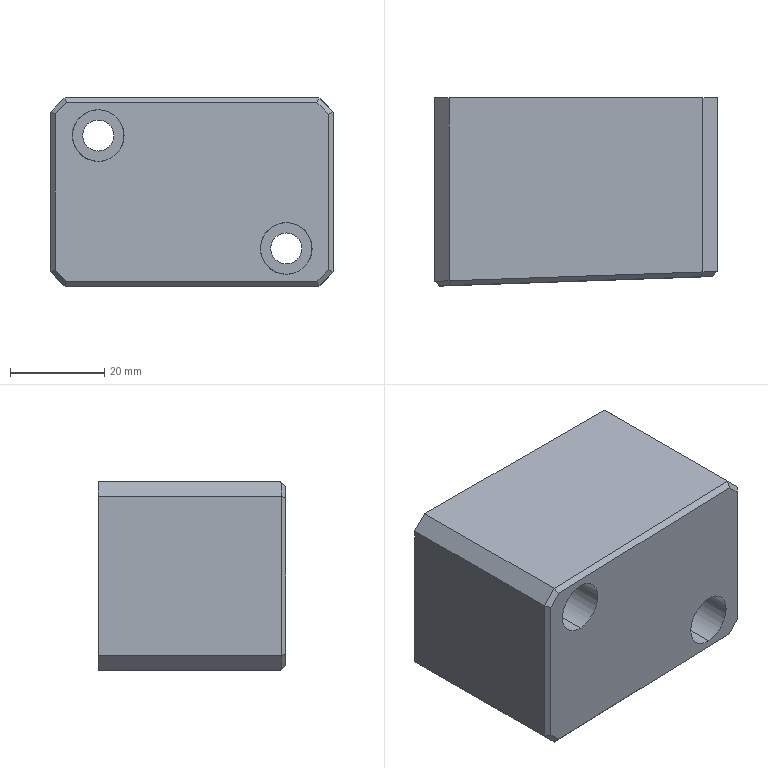Part | SolidWorks | features HoleWzd 3, Chamfer 2, Extrusion 1 | 1 solid | 36 faces | box 60 x 39.966 x 40 mm | volume 86382 mm3 | plane 20 | cylinder 12 | cone 4 | commonest cylinder face diameters 6.6 x4 8 x4 11 x4
STEP:
#1=CARTESIAN_POINT('',(-27.515,48.13,4.));
#2=VERTEX_POINT('',#1);
#3=CARTESIAN_POINT('',(-27.515,48.13,12.));
#4=VERTEX_POINT('',#3);
#5=CARTESIAN_POINT('',(-27.515,48.13,8.));
#6=DIRECTION('',(0.,1.,0.));
#7=DIRECTION('',(0.,0.,1.));
#8=AXIS2_PLACEMENT_3D('',#5,#6,#7);
#9=CIRCLE('',#8,4.);
#10=EDGE_CURVE('',#2,#4,#9,.T.);
#11=ORIENTED_EDGE('',*,*,#10,.F.);
#12=CARTESIAN_POINT('',(-27.515,60.63,4.));
#13=VERTEX_POINT('',#12);
#14=CARTESIAN_POINT('',(-27.515,60.63,4.));
#15=DIRECTION('',(0.,1.,0.));
#16=VECTOR('',#15,1000.);
#17=LINE('',#14,#16);
#18=EDGE_CURVE('',#2,#13,#17,.T.);
#19=ORIENTED_EDGE('',*,*,#18,.T.);
#20=CARTESIAN_POINT('',(-27.515,60.63,12.));
#21=VERTEX_POINT('',#20);
#22=CARTESIAN_POINT('',(-27.515,60.63,8.));
#23=DIRECTION('',(0.,1.,0.));
#24=DIRECTION('',(0.,0.,1.));
#25=AXIS2_PLACEMENT_3D('',#22,#23,#24);
#26=CIRCLE('',#25,4.);
#27=EDGE_CURVE('',#13,#21,#26,.T.);
#28=ORIENTED_EDGE('',*,*,#27,.T.);
#29=CARTESIAN_POINT('',(-27.515,60.63,12.));
#30=DIRECTION('',(0.,1.,0.));
#31=VECTOR('',#30,1000.);
#32=LINE('',#29,#31);
#33=EDGE_CURVE('',#4,#21,#32,.T.);
#34=ORIENTED_EDGE('',*,*,#33,.F.);
#35=EDGE_LOOP('',(#11,#19,#28,#34));
#36=FACE_OUTER_BOUND('',#35,.T.);
#37=CARTESIAN_POINT('',(-27.515,60.63,8.));
#38=DIRECTION('',(0.,1.,0.));
#39=DIRECTION('',(0.,0.,1.));
#40=AXIS2_PLACEMENT_3D('',#37,#38,#39);
#41=CYLINDRICAL_SURFACE('',#40,4.);
#42=ADVANCED_FACE('',(#36),#41,.F.);
#43=CARTESIAN_POINT('',(-27.515,45.727,8.));
#44=VERTEX_POINT('',#43);
#45=CARTESIAN_POINT('',(-27.515,48.13,12.));
#46=DIRECTION('',(0.,0.515,0.8572));
#47=VECTOR('',#46,1000.);
#48=LINE('',#45,#47);
#49=EDGE_CURVE('',#44,#4,#48,.T.);
#50=ORIENTED_EDGE('',*,*,#49,.F.);
#51=CARTESIAN_POINT('',(-27.515,48.13,4.));
#52=DIRECTION('',(0.,0.515,-0.8572));
#53=VECTOR('',#52,1000.);
#54=LINE('',#51,#53);
#55=EDGE_CURVE('',#44,#2,#54,.T.);
#56=ORIENTED_EDGE('',*,*,#55,.T.);
#57=ORIENTED_EDGE('',*,*,#10,.T.);
#58=EDGE_LOOP('',(#50,#56,#57));
#59=FACE_OUTER_BOUND('',#58,.T.);
#60=CARTESIAN_POINT('',(-27.515,48.13,8.));
#61=DIRECTION('',(0.,1.,0.));
#62=DIRECTION('',(0.,0.,1.));
#63=AXIS2_PLACEMENT_3D('',#60,#61,#62);
#64=CONICAL_SURFACE('',#63,4.,1.03);
#65=ADVANCED_FACE('',(#59),#64,.F.);
#66=CARTESIAN_POINT('',(12.461,48.13,28.));
#67=VERTEX_POINT('',#66);
#68=CARTESIAN_POINT('',(12.461,48.13,36.));
#69=VERTEX_POINT('',#68);
#70=CARTESIAN_POINT('',(12.461,48.13,32.));
#71=DIRECTION('',(0.,1.,0.));
#72=DIRECTION('',(0.,0.,1.));
#73=AXIS2_PLACEMENT_3D('',#70,#71,#72);
#74=CIRCLE('',#73,4.);
#75=EDGE_CURVE('',#67,#69,#74,.T.);
#76=ORIENTED_EDGE('',*,*,#75,.F.);
#77=CARTESIAN_POINT('',(12.461,60.63,28.));
#78=VERTEX_POINT('',#77);
#79=CARTESIAN_POINT('',(12.461,60.63,28.));
#80=DIRECTION('',(0.,1.,0.));
#81=VECTOR('',#80,1000.);
#82=LINE('',#79,#81);
#83=EDGE_CURVE('',#67,#78,#82,.T.);
#84=ORIENTED_EDGE('',*,*,#83,.T.);
#85=CARTESIAN_POINT('',(12.461,60.63,36.));
#86=VERTEX_POINT('',#85);
#87=CARTESIAN_POINT('',(12.461,60.63,32.));
#88=DIRECTION('',(0.,1.,0.));
#89=DIRECTION('',(0.,0.,1.));
#90=AXIS2_PLACEMENT_3D('',#87,#88,#89);
#91=CIRCLE('',#90,4.);
#92=EDGE_CURVE('',#78,#86,#91,.T.);
#93=ORIENTED_EDGE('',*,*,#92,.T.);
#94=CARTESIAN_POINT('',(12.461,60.63,36.));
#95=DIRECTION('',(0.,1.,0.));
#96=VECTOR('',#95,1000.);
#97=LINE('',#94,#96);
#98=EDGE_CURVE('',#69,#86,#97,.T.);
#99=ORIENTED_EDGE('',*,*,#98,.F.);
#100=EDGE_LOOP('',(#76,#84,#93,#99));
#101=FACE_OUTER_BOUND('',#100,.T.);
#102=CARTESIAN_POINT('',(12.461,60.63,32.));
#103=DIRECTION('',(0.,1.,0.));
#104=DIRECTION('',(0.,0.,1.));
#105=AXIS2_PLACEMENT_3D('',#102,#103,#104);
#106=CYLINDRICAL_SURFACE('',#105,4.);
#107=ADVANCED_FACE('',(#101),#106,.F.);
#108=CARTESIAN_POINT('',(12.461,45.727,32.));
#109=VERTEX_POINT('',#108);
#110=CARTESIAN_POINT('',(12.461,48.13,36.));
#111=DIRECTION('',(0.,0.515,0.8572));
#112=VECTOR('',#111,1000.);
#113=LINE('',#110,#112);
#114=EDGE_CURVE('',#109,#69,#113,.T.);
#115=ORIENTED_EDGE('',*,*,#114,.F.);
#116=CARTESIAN_POINT('',(12.461,48.13,28.));
#117=DIRECTION('',(0.,0.515,-0.8572));
#118=VECTOR('',#117,1000.);
#119=LINE('',#116,#118);
#120=EDGE_CURVE('',#109,#67,#119,.T.);
#121=ORIENTED_EDGE('',*,*,#120,.T.);
#122=ORIENTED_EDGE('',*,*,#75,.T.);
#123=EDGE_LOOP('',(#115,#121,#122));
#124=FACE_OUTER_BOUND('',#123,.T.);
#125=CARTESIAN_POINT('',(12.461,48.13,32.));
#126=DIRECTION('',(0.,1.,0.));
#127=DIRECTION('',(0.,0.,1.));
#128=AXIS2_PLACEMENT_3D('',#125,#126,#127);
#129=CONICAL_SURFACE('',#128,4.,1.03);
#130=ADVANCED_FACE('',(#124),#129,.F.);
#131=CARTESIAN_POINT('',(-27.515,20.982,26.5));
#132=VERTEX_POINT('',#131);
#133=CARTESIAN_POINT('',(-27.515,20.982,37.5));
#134=VERTEX_POINT('',#133);
#135=CARTESIAN_POINT('',(-27.515,20.982,26.5));
#136=CARTESIAN_POINT('',(-38.515,20.597,26.5));
#137=CARTESIAN_POINT('',(-38.515,20.597,37.5));
#138=CARTESIAN_POINT('',(-27.515,20.982,37.5));
#139=(BOUNDED_CURVE()B_SPLINE_CURVE(3,(#135,#136,#137,#138),.UNSPECIFIED.,.F.,.F.)B_SPLINE_CURVE_WITH_KNOTS((4,4),(1.571,4.712),.UNSPECIFIED.)CURVE()GEOMETRIC_REPRESENTATION_ITEM()RATIONAL_B_SPLINE_CURVE((1.,0.3333,0.3333,1.))REPRESENTATION_ITEM(''));
#140=EDGE_CURVE('',#132,#134,#139,.T.);
#141=ORIENTED_EDGE('',*,*,#140,.F.);
#142=CARTESIAN_POINT('',(-27.515,40.63,26.5));
#143=VERTEX_POINT('',#142);
#144=CARTESIAN_POINT('',(-27.515,40.63,26.5));
#145=DIRECTION('',(0.,1.,0.));
#146=VECTOR('',#145,1000.);
#147=LINE('',#144,#146);
#148=EDGE_CURVE('',#132,#143,#147,.T.);
#149=ORIENTED_EDGE('',*,*,#148,.T.);
#150=CARTESIAN_POINT('',(-27.515,40.63,37.5));
#151=VERTEX_POINT('',#150);
#152=CARTESIAN_POINT('',(-27.515,40.63,32.));
#153=DIRECTION('',(0.,1.,0.));
#154=DIRECTION('',(0.,0.,1.));
#155=AXIS2_PLACEMENT_3D('',#152,#153,#154);
#156=CIRCLE('',#155,5.5);
#157=EDGE_CURVE('',#143,#151,#156,.T.);
#158=ORIENTED_EDGE('',*,*,#157,.T.);
#159=CARTESIAN_POINT('',(-27.515,40.63,37.5));
#160=DIRECTION('',(0.,1.,0.));
#161=VECTOR('',#160,1000.);
#162=LINE('',#159,#161);
#163=EDGE_CURVE('',#134,#151,#162,.T.);
#164=ORIENTED_EDGE('',*,*,#163,.F.);
#165=EDGE_LOOP('',(#141,#149,#158,#164));
#166=FACE_OUTER_BOUND('',#165,.T.);
#167=CARTESIAN_POINT('',(-27.515,40.63,32.));
#168=DIRECTION('',(0.,1.,0.));
#169=DIRECTION('',(0.,0.,1.));
#170=AXIS2_PLACEMENT_3D('',#167,#168,#169);
#171=CYLINDRICAL_SURFACE('',#170,5.5);
#172=ADVANCED_FACE('',(#166),#171,.F.);
#173=CARTESIAN_POINT('',(12.461,22.378,2.5));
#174=VERTEX_POINT('',#173);
#175=CARTESIAN_POINT('',(12.461,22.378,13.5));
#176=VERTEX_POINT('',#175);
#177=CARTESIAN_POINT('',(12.461,22.378,2.5));
#178=CARTESIAN_POINT('',(1.461,21.993,2.5));
#179=CARTESIAN_POINT('',(1.461,21.993,13.5));
#180=CARTESIAN_POINT('',(12.461,22.378,13.5));
#181=(BOUNDED_CURVE()B_SPLINE_CURVE(3,(#177,#178,#179,#180),.UNSPECIFIED.,.F.,.F.)B_SPLINE_CURVE_WITH_KNOTS((4,4),(1.571,4.712),.UNSPECIFIED.)CURVE()GEOMETRIC_REPRESENTATION_ITEM()RATIONAL_B_SPLINE_CURVE((1.,0.3333,0.3333,1.))REPRESENTATION_ITEM(''));
#182=EDGE_CURVE('',#174,#176,#181,.T.);
#183=ORIENTED_EDGE('',*,*,#182,.F.);
#184=CARTESIAN_POINT('',(12.461,40.63,2.5));
#185=VERTEX_POINT('',#184);
#186=CARTESIAN_POINT('',(12.461,40.63,2.5));
#187=DIRECTION('',(0.,1.,0.));
#188=VECTOR('',#187,1000.);
#189=LINE('',#186,#188);
#190=EDGE_CURVE('',#174,#185,#189,.T.);
#191=ORIENTED_EDGE('',*,*,#190,.T.);
#192=CARTESIAN_POINT('',(12.461,40.63,13.5));
#193=VERTEX_POINT('',#192);
#194=CARTESIAN_POINT('',(12.461,40.63,8.));
#195=DIRECTION('',(0.,1.,0.));
#196=DIRECTION('',(0.,0.,1.));
#197=AXIS2_PLACEMENT_3D('',#194,#195,#196);
#198=CIRCLE('',#197,5.5);
#199=EDGE_CURVE('',#185,#193,#198,.T.);
#200=ORIENTED_EDGE('',*,*,#199,.T.);
#201=CARTESIAN_POINT('',(12.461,40.63,13.5));
#202=DIRECTION('',(0.,1.,0.));
#203=VECTOR('',#202,1000.);
#204=LINE('',#201,#203);
#205=EDGE_CURVE('',#176,#193,#204,.T.);
#206=ORIENTED_EDGE('',*,*,#205,.F.);
#207=EDGE_LOOP('',(#183,#191,#200,#206));
#208=FACE_OUTER_BOUND('',#207,.T.);
#209=CARTESIAN_POINT('',(12.461,40.63,8.));
#210=DIRECTION('',(0.,1.,0.));
#211=DIRECTION('',(0.,0.,1.));
#212=AXIS2_PLACEMENT_3D('',#209,#210,#211);
#213=CYLINDRICAL_SURFACE('',#212,5.5);
#214=ADVANCED_FACE('',(#208),#213,.F.);
#215=CARTESIAN_POINT('',(-27.515,40.63,35.3));
#216=VERTEX_POINT('',#215);
#217=CARTESIAN_POINT('',(-27.515,40.63,28.7));
#218=VERTEX_POINT('',#217);
#219=CARTESIAN_POINT('',(-27.515,40.63,32.));
#220=DIRECTION('',(0.,-1.,0.));
#221=DIRECTION('',(0.,0.,1.));
#222=AXIS2_PLACEMENT_3D('',#219,#220,#221);
#223=CIRCLE('',#222,3.3);
#224=EDGE_CURVE('',#216,#218,#223,.T.);
#225=ORIENTED_EDGE('',*,*,#224,.T.);
#226=CARTESIAN_POINT('',(-27.515,60.63,28.7));
#227=VERTEX_POINT('',#226);
#228=CARTESIAN_POINT('',(-27.515,60.63,28.7));
#229=DIRECTION('',(0.,1.,0.));
#230=VECTOR('',#229,1000.);
#231=LINE('',#228,#230);
#232=EDGE_CURVE('',#218,#227,#231,.T.);
#233=ORIENTED_EDGE('',*,*,#232,.T.);
#234=CARTESIAN_POINT('',(-27.515,60.63,35.3));
#235=VERTEX_POINT('',#234);
#236=CARTESIAN_POINT('',(-27.515,60.63,32.));
#237=DIRECTION('',(0.,1.,0.));
#238=DIRECTION('',(0.,0.,1.));
#239=AXIS2_PLACEMENT_3D('',#236,#237,#238);
#240=CIRCLE('',#239,3.3);
#241=EDGE_CURVE('',#227,#235,#240,.T.);
#242=ORIENTED_EDGE('',*,*,#241,.T.);
#243=CARTESIAN_POINT('',(-27.515,60.63,35.3));
#244=DIRECTION('',(0.,1.,0.));
#245=VECTOR('',#244,1000.);
#246=LINE('',#243,#245);
#247=EDGE_CURVE('',#216,#235,#246,.T.);
#248=ORIENTED_EDGE('',*,*,#247,.F.);
#249=EDGE_LOOP('',(#225,#233,#242,#248));
#250=FACE_OUTER_BOUND('',#249,.T.);
#251=CARTESIAN_POINT('',(-27.515,60.63,32.));
#252=DIRECTION('',(0.,1.,0.));
#253=DIRECTION('',(0.,0.,1.));
#254=AXIS2_PLACEMENT_3D('',#251,#252,#253);
#255=CYLINDRICAL_SURFACE('',#254,3.3);
#256=ADVANCED_FACE('',(#250),#255,.F.);
#257=CARTESIAN_POINT('',(12.461,40.63,11.3));
#258=VERTEX_POINT('',#257);
#259=CARTESIAN_POINT('',(12.461,40.63,4.7));
#260=VERTEX_POINT('',#259);
#261=CARTESIAN_POINT('',(12.461,40.63,8.));
#262=DIRECTION('',(0.,-1.,0.));
#263=DIRECTION('',(0.,0.,1.));
#264=AXIS2_PLACEMENT_3D('',#261,#262,#263);
#265=CIRCLE('',#264,3.3);
#266=EDGE_CURVE('',#258,#260,#265,.T.);
#267=ORIENTED_EDGE('',*,*,#266,.T.);
#268=CARTESIAN_POINT('',(12.461,60.63,4.7));
#269=VERTEX_POINT('',#268);
#270=CARTESIAN_POINT('',(12.461,60.63,4.7));
#271=DIRECTION('',(0.,1.,0.));
#272=VECTOR('',#271,1000.);
#273=LINE('',#270,#272);
#274=EDGE_CURVE('',#260,#269,#273,.T.);
#275=ORIENTED_EDGE('',*,*,#274,.T.);
#276=CARTESIAN_POINT('',(12.461,60.63,11.3));
#277=VERTEX_POINT('',#276);
#278=CARTESIAN_POINT('',(12.461,60.63,8.));
#279=DIRECTION('',(0.,1.,0.));
#280=DIRECTION('',(0.,0.,1.));
#281=AXIS2_PLACEMENT_3D('',#278,#279,#280);
#282=CIRCLE('',#281,3.3);
#283=EDGE_CURVE('',#269,#277,#282,.T.);
#284=ORIENTED_EDGE('',*,*,#283,.T.);
#285=CARTESIAN_POINT('',(12.461,60.63,11.3));
#286=DIRECTION('',(0.,1.,0.));
#287=VECTOR('',#286,1000.);
#288=LINE('',#285,#287);
#289=EDGE_CURVE('',#258,#277,#288,.T.);
#290=ORIENTED_EDGE('',*,*,#289,.F.);
#291=EDGE_LOOP('',(#267,#275,#284,#290));
#292=FACE_OUTER_BOUND('',#291,.T.);
#293=CARTESIAN_POINT('',(12.461,60.63,8.));
#294=DIRECTION('',(0.,1.,0.));
#295=DIRECTION('',(0.,0.,1.));
#296=AXIS2_PLACEMENT_3D('',#293,#294,#295);
#297=CYLINDRICAL_SURFACE('',#296,3.3);
#298=ADVANCED_FACE('',(#292),#297,.F.);
#299=CARTESIAN_POINT('',(-37.581,60.63,3.));
#300=VERTEX_POINT('',#299);
#301=CARTESIAN_POINT('',(-37.581,21.63,3.));
#302=VERTEX_POINT('',#301);
#303=CARTESIAN_POINT('',(-37.581,60.63,3.));
#304=DIRECTION('',(0.,-1.,0.));
#305=VECTOR('',#304,1000.);
#306=LINE('',#303,#305);
#307=EDGE_CURVE('',#300,#302,#306,.T.);
#308=ORIENTED_EDGE('',*,*,#307,.T.);
#309=CARTESIAN_POINT('',(-37.581,21.63,3.));
#310=VERTEX_POINT('',#309);
#311=CARTESIAN_POINT('',(-37.581,11.958,16.345));
#312=DIRECTION('',(0.,-0.5869,0.8097));
#313=VECTOR('',#312,1000.);
#314=LINE('',#311,#313);
#315=EDGE_CURVE('',#302,#310,#314,.T.);
#316=ORIENTED_EDGE('',*,*,#315,.T.);
#317=CARTESIAN_POINT('',(-37.581,21.63,37.));
#318=VERTEX_POINT('',#317);
#319=CARTESIAN_POINT('',(-37.581,21.63,40.));
#320=DIRECTION('',(0.,0.,1.));
#321=VECTOR('',#320,1000.);
#322=LINE('',#319,#321);
#323=EDGE_CURVE('',#310,#318,#322,.T.);
#324=ORIENTED_EDGE('',*,*,#323,.T.);
#325=CARTESIAN_POINT('',(-37.581,21.63,37.));
#326=VERTEX_POINT('',#325);
#327=CARTESIAN_POINT('',(-37.581,21.696,37.091));
#328=DIRECTION('',(0.,0.5869,0.8097));
#329=VECTOR('',#328,1000.);
#330=LINE('',#327,#329);
#331=EDGE_CURVE('',#318,#326,#330,.T.);
#332=ORIENTED_EDGE('',*,*,#331,.T.);
#333=CARTESIAN_POINT('',(-37.581,60.63,37.));
#334=VERTEX_POINT('',#333);
#335=CARTESIAN_POINT('',(-37.581,60.63,37.));
#336=DIRECTION('',(0.,1.,0.));
#337=VECTOR('',#336,1000.);
#338=LINE('',#335,#337);
#339=EDGE_CURVE('',#326,#334,#338,.T.);
#340=ORIENTED_EDGE('',*,*,#339,.T.);
#341=CARTESIAN_POINT('',(-37.581,60.63,40.));
#342=DIRECTION('',(0.,0.,-1.));
#343=VECTOR('',#342,1000.);
#344=LINE('',#341,#343);
#345=EDGE_CURVE('',#334,#300,#344,.T.);
#346=ORIENTED_EDGE('',*,*,#345,.T.);
#347=EDGE_LOOP('',(#308,#316,#324,#332,#340,#346));
#348=FACE_OUTER_BOUND('',#347,.T.);
#349=CARTESIAN_POINT('',(-37.581,60.63,40.));
#350=DIRECTION('',(1.,0.,0.));
#351=DIRECTION('',(0.,1.,0.));
#352=AXIS2_PLACEMENT_3D('',#349,#350,#351);
#353=PLANE('',#352);
#354=ADVANCED_FACE('',(#348),#353,.F.);
#355=CARTESIAN_POINT('',(-27.515,20.982,37.5));
#356=CARTESIAN_POINT('',(-16.515,21.366,37.5));
#357=CARTESIAN_POINT('',(-16.515,21.366,26.5));
#358=CARTESIAN_POINT('',(-27.515,20.982,26.5));
#359=(BOUNDED_CURVE()B_SPLINE_CURVE(3,(#355,#356,#357,#358),.UNSPECIFIED.,.F.,.T.)B_SPLINE_CURVE_WITH_KNOTS((4,4),(4.712,7.854),.UNSPECIFIED.)CURVE()GEOMETRIC_REPRESENTATION_ITEM()RATIONAL_B_SPLINE_CURVE((1.,0.3333,0.3333,1.))REPRESENTATION_ITEM(''));
#360=EDGE_CURVE('',#134,#132,#359,.T.);
#361=ORIENTED_EDGE('',*,*,#360,.T.);
#362=ORIENTED_EDGE('',*,*,#140,.T.);
#363=EDGE_LOOP('',(#361,#362));
#364=FACE_BOUND('',#363,.T.);
#365=CARTESIAN_POINT('',(12.461,22.378,13.5));
#366=CARTESIAN_POINT('',(23.461,22.762,13.5));
#367=CARTESIAN_POINT('',(23.461,22.762,2.5));
#368=CARTESIAN_POINT('',(12.461,22.378,2.5));
#369=(BOUNDED_CURVE()B_SPLINE_CURVE(3,(#365,#366,#367,#368),.UNSPECIFIED.,.F.,.T.)B_SPLINE_CURVE_WITH_KNOTS((4,4),(4.712,7.854),.UNSPECIFIED.)CURVE()GEOMETRIC_REPRESENTATION_ITEM()RATIONAL_B_SPLINE_CURVE((1.,0.3333,0.3333,1.))REPRESENTATION_ITEM(''));
#370=EDGE_CURVE('',#176,#174,#369,.T.);
#371=ORIENTED_EDGE('',*,*,#370,.T.);
#372=ORIENTED_EDGE('',*,*,#182,.T.);
#373=EDGE_LOOP('',(#371,#372));
#374=FACE_BOUND('',#373,.T.);
#375=CARTESIAN_POINT('',(21.419,22.69,3.451));
#376=VERTEX_POINT('',#375);
#377=CARTESIAN_POINT('',(21.419,22.69,36.549));
#378=VERTEX_POINT('',#377);
#379=CARTESIAN_POINT('',(21.419,22.69,40.));
#380=DIRECTION('',(0.,0.,1.));
#381=VECTOR('',#380,1000.);
#382=LINE('',#379,#381);
#383=EDGE_CURVE('',#376,#378,#382,.T.);
#384=ORIENTED_EDGE('',*,*,#383,.T.);
#385=CARTESIAN_POINT('',(18.969,22.605,39.));
#386=VERTEX_POINT('',#385);
#387=CARTESIAN_POINT('',(18.694,22.595,39.275));
#388=DIRECTION('',(-0.7069,-0.02469,0.7069));
#389=VECTOR('',#388,1000.);
#390=LINE('',#387,#389);
#391=EDGE_CURVE('',#378,#386,#390,.T.);
#392=ORIENTED_EDGE('',*,*,#391,.T.);
#393=CARTESIAN_POINT('',(-34.201,20.748,39.));
#394=VERTEX_POINT('',#393);
#395=CARTESIAN_POINT('',(-34.581,20.735,39.));
#396=DIRECTION('',(-0.9994,-0.0349,0.));
#397=VECTOR('',#396,1000.);
#398=LINE('',#395,#397);
#399=EDGE_CURVE('',#386,#394,#398,.T.);
#400=ORIENTED_EDGE('',*,*,#399,.T.);
#401=CARTESIAN_POINT('',(-36.615,20.664,36.586));
#402=VERTEX_POINT('',#401);
#403=CARTESIAN_POINT('',(-36.892,20.654,36.31));
#404=DIRECTION('',(-0.7069,-0.02469,-0.7069));
#405=VECTOR('',#404,1000.);
#406=LINE('',#403,#405);
#407=EDGE_CURVE('',#394,#402,#406,.T.);
#408=ORIENTED_EDGE('',*,*,#407,.T.);
#409=CARTESIAN_POINT('',(-36.615,20.664,3.414));
#410=VERTEX_POINT('',#409);
#411=CARTESIAN_POINT('',(-36.615,20.664,40.));
#412=DIRECTION('',(0.,0.,-1.));
#413=VECTOR('',#412,1000.);
#414=LINE('',#411,#413);
#415=EDGE_CURVE('',#402,#410,#414,.T.);
#416=ORIENTED_EDGE('',*,*,#415,.T.);
#417=CARTESIAN_POINT('',(-34.201,20.748,1.));
#418=VERTEX_POINT('',#417);
#419=CARTESIAN_POINT('',(-33.892,20.759,0.6905));
#420=DIRECTION('',(0.7069,0.02469,-0.7069));
#421=VECTOR('',#420,1000.);
#422=LINE('',#419,#421);
#423=EDGE_CURVE('',#410,#418,#422,.T.);
#424=ORIENTED_EDGE('',*,*,#423,.T.);
#425=CARTESIAN_POINT('',(18.969,22.605,1.));
#426=VERTEX_POINT('',#425);
#427=CARTESIAN_POINT('',(-37.581,20.63,1.));
#428=DIRECTION('',(0.9994,0.0349,0.));
#429=VECTOR('',#428,1000.);
#430=LINE('',#427,#429);
#431=EDGE_CURVE('',#418,#426,#430,.T.);
#432=ORIENTED_EDGE('',*,*,#431,.T.);
#433=CARTESIAN_POINT('',(21.694,22.7,3.725));
#434=DIRECTION('',(0.7069,0.02469,0.7069));
#435=VECTOR('',#434,1000.);
#436=LINE('',#433,#435);
#437=EDGE_CURVE('',#426,#376,#436,.T.);
#438=ORIENTED_EDGE('',*,*,#437,.T.);
#439=EDGE_LOOP('',(#384,#392,#400,#408,#416,#424,#432,#438));
#440=FACE_OUTER_BOUND('',#439,.T.);
#441=CARTESIAN_POINT('',(-37.581,20.63,40.));
#442=DIRECTION('',(-0.0349,0.9994,0.));
#443=DIRECTION('',(-0.9994,-0.0349,0.));
#444=AXIS2_PLACEMENT_3D('',#441,#442,#443);
#445=PLANE('',#444);
#446=ADVANCED_FACE('',(#364,#374,#440),#445,.F.);
#447=CARTESIAN_POINT('',(22.419,60.63,37.));
#448=VERTEX_POINT('',#447);
#449=CARTESIAN_POINT('',(22.419,23.762,37.));
#450=VERTEX_POINT('',#449);
#451=CARTESIAN_POINT('',(22.419,22.725,37.));
#452=DIRECTION('',(0.,-1.,0.));
#453=VECTOR('',#452,1000.);
#454=LINE('',#451,#453);
#455=EDGE_CURVE('',#448,#450,#454,.T.);
#456=ORIENTED_EDGE('',*,*,#455,.T.);
#457=CARTESIAN_POINT('',(22.419,23.762,3.));
#458=VERTEX_POINT('',#457);
#459=CARTESIAN_POINT('',(22.419,23.762,40.));
#460=DIRECTION('',(0.,0.,-1.));
#461=VECTOR('',#460,1000.);
#462=LINE('',#459,#461);
#463=EDGE_CURVE('',#450,#458,#462,.T.);
#464=ORIENTED_EDGE('',*,*,#463,.T.);
#465=CARTESIAN_POINT('',(22.419,60.63,3.));
#466=VERTEX_POINT('',#465);
#467=CARTESIAN_POINT('',(22.419,60.63,3.));
#468=DIRECTION('',(0.,1.,0.));
#469=VECTOR('',#468,1000.);
#470=LINE('',#467,#469);
#471=EDGE_CURVE('',#458,#466,#470,.T.);
#472=ORIENTED_EDGE('',*,*,#471,.T.);
#473=CARTESIAN_POINT('',(22.419,60.63,40.));
#474=DIRECTION('',(0.,0.,-1.));
#475=VECTOR('',#474,1000.);
#476=LINE('',#473,#475);
#477=EDGE_CURVE('',#448,#466,#476,.T.);
#478=ORIENTED_EDGE('',*,*,#477,.F.);
#479=EDGE_LOOP('',(#456,#464,#472,#478));
#480=FACE_OUTER_BOUND('',#479,.T.);
#481=CARTESIAN_POINT('',(22.419,60.63,40.));
#482=DIRECTION('',(-1.,0.,0.));
#483=DIRECTION('',(0.,-1.,0.));
#484=AXIS2_PLACEMENT_3D('',#481,#482,#483);
#485=PLANE('',#484);
#486=ADVANCED_FACE('',(#480),#485,.F.);
#487=CARTESIAN_POINT('',(-27.515,60.63,8.));
#488=DIRECTION('',(0.,1.,0.));
#489=DIRECTION('',(0.,0.,1.));
#490=AXIS2_PLACEMENT_3D('',#487,#488,#489);
#491=CIRCLE('',#490,4.);
#492=EDGE_CURVE('',#21,#13,#491,.T.);
#493=ORIENTED_EDGE('',*,*,#492,.F.);
#494=ORIENTED_EDGE('',*,*,#27,.F.);
#495=EDGE_LOOP('',(#493,#494));
#496=FACE_BOUND('',#495,.T.);
#497=CARTESIAN_POINT('',(12.461,60.63,32.));
#498=DIRECTION('',(0.,1.,0.));
#499=DIRECTION('',(0.,0.,1.));
#500=AXIS2_PLACEMENT_3D('',#497,#498,#499);
#501=CIRCLE('',#500,4.);
#502=EDGE_CURVE('',#86,#78,#501,.T.);
#503=ORIENTED_EDGE('',*,*,#502,.F.);
#504=ORIENTED_EDGE('',*,*,#92,.F.);
#505=EDGE_LOOP('',(#503,#504));
#506=FACE_BOUND('',#505,.T.);
#507=CARTESIAN_POINT('',(-27.515,60.63,32.));
#508=DIRECTION('',(0.,1.,0.));
#509=DIRECTION('',(0.,0.,1.));
#510=AXIS2_PLACEMENT_3D('',#507,#508,#509);
#511=CIRCLE('',#510,3.3);
#512=EDGE_CURVE('',#235,#227,#511,.T.);
#513=ORIENTED_EDGE('',*,*,#512,.F.);
#514=ORIENTED_EDGE('',*,*,#241,.F.);
#515=EDGE_LOOP('',(#513,#514));
#516=FACE_BOUND('',#515,.T.);
#517=CARTESIAN_POINT('',(12.461,60.63,8.));
#518=DIRECTION('',(0.,1.,0.));
#519=DIRECTION('',(0.,0.,1.));
#520=AXIS2_PLACEMENT_3D('',#517,#518,#519);
#521=CIRCLE('',#520,3.3);
#522=EDGE_CURVE('',#277,#269,#521,.T.);
#523=ORIENTED_EDGE('',*,*,#522,.F.);
#524=ORIENTED_EDGE('',*,*,#283,.F.);
#525=EDGE_LOOP('',(#523,#524));
#526=FACE_BOUND('',#525,.T.);
#527=CARTESIAN_POINT('',(19.419,60.63,0.));
#528=VERTEX_POINT('',#527);
#529=CARTESIAN_POINT('',(-34.581,60.63,0.));
#530=VERTEX_POINT('',#529);
#531=CARTESIAN_POINT('',(-37.581,60.63,0.));
#532=DIRECTION('',(-1.,0.,0.));
#533=VECTOR('',#532,1000.);
#534=LINE('',#531,#533);
#535=EDGE_CURVE('',#528,#530,#534,.T.);
#536=ORIENTED_EDGE('',*,*,#535,.T.);
#537=CARTESIAN_POINT('',(-37.581,60.63,3.));
#538=DIRECTION('',(-0.7071,0.,0.7071));
#539=VECTOR('',#538,1000.);
#540=LINE('',#537,#539);
#541=EDGE_CURVE('',#530,#300,#540,.T.);
#542=ORIENTED_EDGE('',*,*,#541,.T.);
#543=ORIENTED_EDGE('',*,*,#345,.F.);
#544=CARTESIAN_POINT('',(-34.581,60.63,40.));
#545=VERTEX_POINT('',#544);
#546=CARTESIAN_POINT('',(-34.581,60.63,40.));
#547=DIRECTION('',(0.7071,0.,0.7071));
#548=VECTOR('',#547,1000.);
#549=LINE('',#546,#548);
#550=EDGE_CURVE('',#334,#545,#549,.T.);
#551=ORIENTED_EDGE('',*,*,#550,.T.);
#552=CARTESIAN_POINT('',(19.419,60.63,40.));
#553=VERTEX_POINT('',#552);
#554=CARTESIAN_POINT('',(-37.581,60.63,40.));
#555=DIRECTION('',(-1.,0.,0.));
#556=VECTOR('',#555,1000.);
#557=LINE('',#554,#556);
#558=EDGE_CURVE('',#553,#545,#557,.T.);
#559=ORIENTED_EDGE('',*,*,#558,.F.);
#560=CARTESIAN_POINT('',(19.419,60.63,40.));
#561=DIRECTION('',(0.7071,0.,-0.7071));
#562=VECTOR('',#561,1000.);
#563=LINE('',#560,#562);
#564=EDGE_CURVE('',#553,#448,#563,.T.);
#565=ORIENTED_EDGE('',*,*,#564,.T.);
#566=ORIENTED_EDGE('',*,*,#477,.T.);
#567=CARTESIAN_POINT('',(22.419,60.63,3.));
#568=DIRECTION('',(-0.7071,0.,-0.7071));
#569=VECTOR('',#568,1000.);
#570=LINE('',#567,#569);
#571=EDGE_CURVE('',#466,#528,#570,.T.);
#572=ORIENTED_EDGE('',*,*,#571,.T.);
#573=EDGE_LOOP('',(#536,#542,#543,#551,#559,#565,#566,#572));
#574=FACE_OUTER_BOUND('',#573,.T.);
#575=CARTESIAN_POINT('',(-37.581,60.63,40.));
#576=DIRECTION('',(0.,-1.,0.));
#577=DIRECTION('',(1.,0.,0.));
#578=AXIS2_PLACEMENT_3D('',#575,#576,#577);
#579=PLANE('',#578);
#580=ADVANCED_FACE('',(#496,#506,#516,#526,#574),#579,.F.);
#581=CARTESIAN_POINT('',(-34.581,21.735,40.));
#582=VERTEX_POINT('',#581);
#583=CARTESIAN_POINT('',(-34.581,20.63,40.));
#584=DIRECTION('',(0.,-1.,0.));
#585=VECTOR('',#584,1000.);
#586=LINE('',#583,#585);
#587=EDGE_CURVE('',#545,#582,#586,.T.);
#588=ORIENTED_EDGE('',*,*,#587,.T.);
#589=CARTESIAN_POINT('',(19.419,23.621,40.));
#590=VERTEX_POINT('',#589);
#591=CARTESIAN_POINT('',(19.384,23.62,40.));
#592=DIRECTION('',(0.9994,0.0349,0.));
#593=VECTOR('',#592,1000.);
#594=LINE('',#591,#593);
#595=EDGE_CURVE('',#582,#590,#594,.T.);
#596=ORIENTED_EDGE('',*,*,#595,.T.);
#597=CARTESIAN_POINT('',(19.419,60.63,40.));
#598=DIRECTION('',(0.,1.,0.));
#599=VECTOR('',#598,1000.);
#600=LINE('',#597,#599);
#601=EDGE_CURVE('',#590,#553,#600,.T.);
#602=ORIENTED_EDGE('',*,*,#601,.T.);
#603=ORIENTED_EDGE('',*,*,#558,.T.);
#604=EDGE_LOOP('',(#588,#596,#602,#603));
#605=FACE_OUTER_BOUND('',#604,.T.);
#606=CARTESIAN_POINT('',(0.,0.,40.));
#607=DIRECTION('',(0.,0.,1.));
#608=DIRECTION('',(1.,0.,0.));
#609=AXIS2_PLACEMENT_3D('',#606,#607,#608);
#610=PLANE('',#609);
#611=ADVANCED_FACE('',(#605),#610,.T.);
#612=CARTESIAN_POINT('',(19.419,23.621,0.));
#613=VERTEX_POINT('',#612);
#614=CARTESIAN_POINT('',(19.419,0.,0.));
#615=DIRECTION('',(0.,-1.,0.));
#616=VECTOR('',#615,1000.);
#617=LINE('',#614,#616);
#618=EDGE_CURVE('',#528,#613,#617,.T.);
#619=ORIENTED_EDGE('',*,*,#618,.T.);
#620=CARTESIAN_POINT('',(-34.581,21.735,0.));
#621=VERTEX_POINT('',#620);
#622=CARTESIAN_POINT('',(-0.8002,22.915,0.));
#623=DIRECTION('',(-0.9994,-0.0349,0.));
#624=VECTOR('',#623,1000.);
#625=LINE('',#622,#624);
#626=EDGE_CURVE('',#613,#621,#625,.T.);
#627=ORIENTED_EDGE('',*,*,#626,.T.);
#628=CARTESIAN_POINT('',(-34.581,0.,0.));
#629=DIRECTION('',(0.,1.,0.));
#630=VECTOR('',#629,1000.);
#631=LINE('',#628,#630);
#632=EDGE_CURVE('',#621,#530,#631,.T.);
#633=ORIENTED_EDGE('',*,*,#632,.T.);
#634=ORIENTED_EDGE('',*,*,#535,.F.);
#635=EDGE_LOOP('',(#619,#627,#633,#634));
#636=FACE_OUTER_BOUND('',#635,.T.);
#637=CARTESIAN_POINT('',(0.,0.,0.));
#638=DIRECTION('',(0.,0.,1.));
#639=DIRECTION('',(1.,0.,0.));
#640=AXIS2_PLACEMENT_3D('',#637,#638,#639);
#641=PLANE('',#640);
#642=ADVANCED_FACE('',(#636),#641,.F.);
#643=ORIENTED_EDGE('',*,*,#632,.F.);
#644=CARTESIAN_POINT('',(-34.582,21.735,0.0003045));
#645=VERTEX_POINT('',#644);
#646=CARTESIAN_POINT('',(-23.425,33.288,-11.157));
#647=DIRECTION('',(-0.5705,-0.5908,0.5705));
#648=VECTOR('',#647,1000.);
#649=LINE('',#646,#648);
#650=EDGE_CURVE('',#621,#645,#649,.T.);
#651=ORIENTED_EDGE('',*,*,#650,.T.);
#652=CARTESIAN_POINT('',(-37.599,21.63,3.017));
#653=DIRECTION('',(-0.7069,-0.02469,0.7069));
#654=VECTOR('',#653,1000.);
#655=LINE('',#652,#654);
#656=EDGE_CURVE('',#645,#302,#655,.T.);
#657=ORIENTED_EDGE('',*,*,#656,.T.);
#658=ORIENTED_EDGE('',*,*,#307,.F.);
#659=ORIENTED_EDGE('',*,*,#541,.F.);
#660=EDGE_LOOP('',(#643,#651,#657,#658,#659));
#661=FACE_OUTER_BOUND('',#660,.T.);
#662=CARTESIAN_POINT('',(-37.581,60.63,3.));
#663=DIRECTION('',(0.7071,0.,0.7071));
#664=DIRECTION('',(0.,-1.,0.));
#665=AXIS2_PLACEMENT_3D('',#662,#663,#664);
#666=PLANE('',#665);
#667=ADVANCED_FACE('',(#661),#666,.F.);
#668=ORIENTED_EDGE('',*,*,#471,.F.);
#669=CARTESIAN_POINT('',(22.383,23.724,2.965));
#670=VERTEX_POINT('',#669);
#671=CARTESIAN_POINT('',(34.97,37.222,15.551));
#672=DIRECTION('',(-0.5634,-0.6042,-0.5634));
#673=VECTOR('',#672,1000.);
#674=LINE('',#671,#673);
#675=EDGE_CURVE('',#458,#670,#674,.T.);
#676=ORIENTED_EDGE('',*,*,#675,.T.);
#677=CARTESIAN_POINT('',(19.419,23.621,0.0003045));
#678=VERTEX_POINT('',#677);
#679=CARTESIAN_POINT('',(19.401,23.62,-0.01746));
#680=DIRECTION('',(-0.7069,-0.02469,-0.7069));
#681=VECTOR('',#680,1000.);
#682=LINE('',#679,#681);
#683=EDGE_CURVE('',#670,#678,#682,.T.);
#684=ORIENTED_EDGE('',*,*,#683,.T.);
#685=CARTESIAN_POINT('',(9.278,33.414,-10.141));
#686=DIRECTION('',(-0.584,0.5639,-0.584));
#687=VECTOR('',#686,1000.);
#688=LINE('',#685,#687);
#689=EDGE_CURVE('',#678,#613,#688,.T.);
#690=ORIENTED_EDGE('',*,*,#689,.T.);
#691=ORIENTED_EDGE('',*,*,#618,.F.);
#692=ORIENTED_EDGE('',*,*,#571,.F.);
#693=EDGE_LOOP('',(#668,#676,#684,#690,#691,#692));
#694=FACE_OUTER_BOUND('',#693,.T.);
#695=CARTESIAN_POINT('',(22.419,60.63,3.));
#696=DIRECTION('',(-0.7071,0.,0.7071));
#697=DIRECTION('',(0.,1.,0.));
#698=AXIS2_PLACEMENT_3D('',#695,#696,#697);
#699=PLANE('',#698);
#700=ADVANCED_FACE('',(#694),#699,.F.);
#701=CARTESIAN_POINT('',(19.419,23.621,40.));
#702=VERTEX_POINT('',#701);
#703=CARTESIAN_POINT('',(22.383,23.724,37.035));
#704=VERTEX_POINT('',#703);
#705=CARTESIAN_POINT('',(22.401,23.725,37.017));
#706=DIRECTION('',(0.7069,0.02469,-0.7069));
#707=VECTOR('',#706,1000.);
#708=LINE('',#705,#707);
#709=EDGE_CURVE('',#702,#704,#708,.T.);
#710=ORIENTED_EDGE('',*,*,#709,.T.);
#711=CARTESIAN_POINT('',(12.424,13.045,46.994));
#712=DIRECTION('',(0.5634,0.6042,-0.5634));
#713=VECTOR('',#712,1000.);
#714=LINE('',#711,#713);
#715=EDGE_CURVE('',#704,#450,#714,.T.);
#716=ORIENTED_EDGE('',*,*,#715,.T.);
#717=ORIENTED_EDGE('',*,*,#455,.F.);
#718=ORIENTED_EDGE('',*,*,#564,.F.);
#719=ORIENTED_EDGE('',*,*,#601,.F.);
#720=CARTESIAN_POINT('',(27.197,16.11,32.222));
#721=DIRECTION('',(0.584,-0.5639,-0.584));
#722=VECTOR('',#721,1000.);
#723=LINE('',#720,#722);
#724=EDGE_CURVE('',#590,#702,#723,.T.);
#725=ORIENTED_EDGE('',*,*,#724,.T.);
#726=EDGE_LOOP('',(#710,#716,#717,#718,#719,#725));
#727=FACE_OUTER_BOUND('',#726,.T.);
#728=CARTESIAN_POINT('',(19.419,0.,40.));
#729=DIRECTION('',(0.7071,0.,0.7071));
#730=DIRECTION('',(0.,-1.,0.));
#731=AXIS2_PLACEMENT_3D('',#728,#729,#730);
#732=PLANE('',#731);
#733=ADVANCED_FACE('',(#727),#732,.T.);
#734=ORIENTED_EDGE('',*,*,#339,.F.);
#735=CARTESIAN_POINT('',(-34.582,21.735,40.));
#736=VERTEX_POINT('',#735);
#737=CARTESIAN_POINT('',(-34.599,21.735,39.983));
#738=DIRECTION('',(0.7069,0.02469,0.7069));
#739=VECTOR('',#738,1000.);
#740=LINE('',#737,#739);
#741=EDGE_CURVE('',#326,#736,#740,.T.);
#742=ORIENTED_EDGE('',*,*,#741,.T.);
#743=CARTESIAN_POINT('',(-41.907,14.149,32.674));
#744=DIRECTION('',(0.5705,0.5908,0.5705));
#745=VECTOR('',#744,1000.);
#746=LINE('',#743,#745);
#747=EDGE_CURVE('',#736,#582,#746,.T.);
#748=ORIENTED_EDGE('',*,*,#747,.T.);
#749=ORIENTED_EDGE('',*,*,#587,.F.);
#750=ORIENTED_EDGE('',*,*,#550,.F.);
#751=EDGE_LOOP('',(#734,#742,#748,#749,#750));
#752=FACE_OUTER_BOUND('',#751,.T.);
#753=CARTESIAN_POINT('',(-34.581,0.,40.));
#754=DIRECTION('',(-0.7071,0.,0.7071));
#755=DIRECTION('',(0.,1.,0.));
#756=AXIS2_PLACEMENT_3D('',#753,#754,#755);
#757=PLANE('',#756);
#758=ADVANCED_FACE('',(#752),#757,.T.);
#759=ORIENTED_EDGE('',*,*,#315,.F.);
#760=ORIENTED_EDGE('',*,*,#656,.F.);
#761=CARTESIAN_POINT('',(-31.715,14.297,7.534));
#762=DIRECTION('',(-0.2614,0.6782,-0.6869));
#763=VECTOR('',#762,1000.);
#764=LINE('',#761,#763);
#765=EDGE_CURVE('',#418,#645,#764,.T.);
#766=ORIENTED_EDGE('',*,*,#765,.F.);
#767=ORIENTED_EDGE('',*,*,#423,.F.);
#768=CARTESIAN_POINT('',(-29.444,13.493,6.482));
#769=DIRECTION('',(0.6768,-0.6768,0.2896));
#770=VECTOR('',#769,1000.);
#771=LINE('',#768,#770);
#772=EDGE_CURVE('',#310,#410,#771,.T.);
#773=ORIENTED_EDGE('',*,*,#772,.F.);
#774=EDGE_LOOP('',(#759,#760,#766,#767,#773));
#775=FACE_OUTER_BOUND('',#774,.T.);
#776=CARTESIAN_POINT('',(-55.381,20.008,22.179));
#777=DIRECTION('',(0.4877,0.7069,0.5123));
#778=DIRECTION('',(0.7069,0.02469,-0.7069));
#779=AXIS2_PLACEMENT_3D('',#776,#777,#778);
#780=PLANE('',#779);
#781=ADVANCED_FACE('',(#775),#780,.F.);
#782=ORIENTED_EDGE('',*,*,#626,.F.);
#783=ORIENTED_EDGE('',*,*,#689,.F.);
#784=CARTESIAN_POINT('',(13.432,10.113,13.291));
#785=DIRECTION('',(0.3012,0.6797,-0.6688));
#786=VECTOR('',#785,1000.);
#787=LINE('',#784,#786);
#788=EDGE_CURVE('',#426,#678,#787,.T.);
#789=ORIENTED_EDGE('',*,*,#788,.F.);
#790=ORIENTED_EDGE('',*,*,#431,.F.);
#791=ORIENTED_EDGE('',*,*,#765,.T.);
#792=ORIENTED_EDGE('',*,*,#650,.F.);
#793=EDGE_LOOP('',(#782,#783,#789,#790,#791,#792));
#794=FACE_OUTER_BOUND('',#793,.T.);
#795=CARTESIAN_POINT('',(-37.581,20.63,1.));
#796=DIRECTION('',(-0.02468,0.7067,0.7071));
#797=DIRECTION('',(0.9994,0.0349,0.));
#798=AXIS2_PLACEMENT_3D('',#795,#796,#797);
#799=PLANE('',#798);
#800=ADVANCED_FACE('',(#794),#799,.F.);
#801=ORIENTED_EDGE('',*,*,#772,.T.);
#802=ORIENTED_EDGE('',*,*,#415,.F.);
#803=CARTESIAN_POINT('',(-36.314,20.363,36.457));
#804=DIRECTION('',(0.6768,-0.6768,-0.2896));
#805=VECTOR('',#804,1000.);
#806=LINE('',#803,#805);
#807=EDGE_CURVE('',#318,#402,#806,.T.);
#808=ORIENTED_EDGE('',*,*,#807,.F.);
#809=ORIENTED_EDGE('',*,*,#323,.F.);
#810=EDGE_LOOP('',(#801,#802,#808,#809));
#811=FACE_OUTER_BOUND('',#810,.T.);
#812=CARTESIAN_POINT('',(-36.615,20.664,40.));
#813=DIRECTION('',(0.7071,0.7071,0.));
#814=DIRECTION('',(0.,0.,-1.));
#815=AXIS2_PLACEMENT_3D('',#812,#813,#814);
#816=PLANE('',#815);
#817=ADVANCED_FACE('',(#811),#816,.F.);
#818=ORIENTED_EDGE('',*,*,#788,.T.);
#819=ORIENTED_EDGE('',*,*,#683,.F.);
#820=CARTESIAN_POINT('',(18.921,20.011,4.709));
#821=DIRECTION('',(0.645,0.6917,-0.325));
#822=VECTOR('',#821,1000.);
#823=LINE('',#820,#822);
#824=EDGE_CURVE('',#376,#670,#823,.T.);
#825=ORIENTED_EDGE('',*,*,#824,.F.);
#826=ORIENTED_EDGE('',*,*,#437,.F.);
#827=EDGE_LOOP('',(#818,#819,#825,#826));
#828=FACE_OUTER_BOUND('',#827,.T.);
#829=CARTESIAN_POINT('',(10.164,22.297,-7.804));
#830=DIRECTION('',(-0.5123,0.7069,0.4877));
#831=DIRECTION('',(0.7069,0.02469,0.7069));
#832=AXIS2_PLACEMENT_3D('',#829,#830,#831);
#833=PLANE('',#832);
#834=ADVANCED_FACE('',(#828),#833,.F.);
#835=ORIENTED_EDGE('',*,*,#807,.T.);
#836=ORIENTED_EDGE('',*,*,#407,.F.);
#837=CARTESIAN_POINT('',(-32.483,16.29,34.484));
#838=DIRECTION('',(0.2614,-0.6782,-0.6869));
#839=VECTOR('',#838,1000.);
#840=LINE('',#837,#839);
#841=EDGE_CURVE('',#736,#394,#840,.T.);
#842=ORIENTED_EDGE('',*,*,#841,.F.);
#843=ORIENTED_EDGE('',*,*,#741,.F.);
#844=ORIENTED_EDGE('',*,*,#331,.F.);
#845=EDGE_LOOP('',(#835,#836,#842,#843,#844));
#846=FACE_OUTER_BOUND('',#845,.T.);
#847=CARTESIAN_POINT('',(-35.393,20.706,37.809));
#848=DIRECTION('',(-0.4877,-0.7069,0.5123));
#849=DIRECTION('',(0.7069,0.02469,0.7069));
#850=AXIS2_PLACEMENT_3D('',#847,#848,#849);
#851=PLANE('',#850);
#852=ADVANCED_FACE('',(#846),#851,.T.);
#853=ORIENTED_EDGE('',*,*,#463,.F.);
#854=ORIENTED_EDGE('',*,*,#715,.F.);
#855=CARTESIAN_POINT('',(23.036,24.425,37.364));
#856=DIRECTION('',(0.645,0.6917,0.325));
#857=VECTOR('',#856,1000.);
#858=LINE('',#855,#857);
#859=EDGE_CURVE('',#378,#704,#858,.T.);
#860=ORIENTED_EDGE('',*,*,#859,.F.);
#861=ORIENTED_EDGE('',*,*,#383,.F.);
#862=ORIENTED_EDGE('',*,*,#824,.T.);
#863=ORIENTED_EDGE('',*,*,#675,.F.);
#864=EDGE_LOOP('',(#853,#854,#860,#861,#862,#863));
#865=FACE_OUTER_BOUND('',#864,.T.);
#866=CARTESIAN_POINT('',(22.419,23.762,40.));
#867=DIRECTION('',(-0.7314,0.682,0.));
#868=DIRECTION('',(0.,0.,-1.));
#869=AXIS2_PLACEMENT_3D('',#866,#867,#868);
#870=PLANE('',#869);
#871=ADVANCED_FACE('',(#865),#870,.F.);
#872=ORIENTED_EDGE('',*,*,#841,.T.);
#873=ORIENTED_EDGE('',*,*,#399,.F.);
#874=CARTESIAN_POINT('',(17.44,19.155,35.606));
#875=DIRECTION('',(-0.3012,-0.6797,-0.6688));
#876=VECTOR('',#875,1000.);
#877=LINE('',#874,#876);
#878=EDGE_CURVE('',#702,#386,#877,.T.);
#879=ORIENTED_EDGE('',*,*,#878,.F.);
#880=ORIENTED_EDGE('',*,*,#724,.F.);
#881=ORIENTED_EDGE('',*,*,#595,.F.);
#882=ORIENTED_EDGE('',*,*,#747,.F.);
#883=EDGE_LOOP('',(#872,#873,#879,#880,#881,#882));
#884=FACE_OUTER_BOUND('',#883,.T.);
#885=CARTESIAN_POINT('',(-0.8002,22.915,40.));
#886=DIRECTION('',(0.02468,-0.7067,0.7071));
#887=DIRECTION('',(-0.9994,-0.0349,0.));
#888=AXIS2_PLACEMENT_3D('',#885,#886,#887);
#889=PLANE('',#888);
#890=ADVANCED_FACE('',(#884),#889,.T.);
#891=ORIENTED_EDGE('',*,*,#859,.T.);
#892=ORIENTED_EDGE('',*,*,#709,.F.);
#893=ORIENTED_EDGE('',*,*,#878,.T.);
#894=ORIENTED_EDGE('',*,*,#391,.F.);
#895=EDGE_LOOP('',(#891,#892,#893,#894));
#896=FACE_OUTER_BOUND('',#895,.T.);
#897=CARTESIAN_POINT('',(-9.823,21.599,67.792));
#898=DIRECTION('',(0.5123,-0.7069,0.4877));
#899=DIRECTION('',(0.7069,0.02469,-0.7069));
#900=AXIS2_PLACEMENT_3D('',#897,#898,#899);
#901=PLANE('',#900);
#902=ADVANCED_FACE('',(#896),#901,.T.);
#903=ORIENTED_EDGE('',*,*,#274,.F.);
#904=CARTESIAN_POINT('',(12.461,40.63,8.));
#905=DIRECTION('',(0.,-1.,0.));
#906=DIRECTION('',(0.,0.,1.));
#907=AXIS2_PLACEMENT_3D('',#904,#905,#906);
#908=CIRCLE('',#907,3.3);
#909=EDGE_CURVE('',#260,#258,#908,.T.);
#910=ORIENTED_EDGE('',*,*,#909,.T.);
#911=ORIENTED_EDGE('',*,*,#289,.T.);
#912=ORIENTED_EDGE('',*,*,#522,.T.);
#913=EDGE_LOOP('',(#903,#910,#911,#912));
#914=FACE_OUTER_BOUND('',#913,.T.);
#915=CARTESIAN_POINT('',(12.461,60.63,8.));
#916=DIRECTION('',(0.,1.,0.));
#917=DIRECTION('',(0.,0.,1.));
#918=AXIS2_PLACEMENT_3D('',#915,#916,#917);
#919=CYLINDRICAL_SURFACE('',#918,3.3);
#920=ADVANCED_FACE('',(#914),#919,.F.);
#921=ORIENTED_EDGE('',*,*,#232,.F.);
#922=CARTESIAN_POINT('',(-27.515,40.63,32.));
#923=DIRECTION('',(0.,-1.,0.));
#924=DIRECTION('',(0.,0.,1.));
#925=AXIS2_PLACEMENT_3D('',#922,#923,#924);
#926=CIRCLE('',#925,3.3);
#927=EDGE_CURVE('',#218,#216,#926,.T.);
#928=ORIENTED_EDGE('',*,*,#927,.T.);
#929=ORIENTED_EDGE('',*,*,#247,.T.);
#930=ORIENTED_EDGE('',*,*,#512,.T.);
#931=EDGE_LOOP('',(#921,#928,#929,#930));
#932=FACE_OUTER_BOUND('',#931,.T.);
#933=CARTESIAN_POINT('',(-27.515,60.63,32.));
#934=DIRECTION('',(0.,1.,0.));
#935=DIRECTION('',(0.,0.,1.));
#936=AXIS2_PLACEMENT_3D('',#933,#934,#935);
#937=CYLINDRICAL_SURFACE('',#936,3.3);
#938=ADVANCED_FACE('',(#932),#937,.F.);
#939=ORIENTED_EDGE('',*,*,#190,.F.);
#940=ORIENTED_EDGE('',*,*,#370,.F.);
#941=ORIENTED_EDGE('',*,*,#205,.T.);
#942=CARTESIAN_POINT('',(12.461,40.63,8.));
#943=DIRECTION('',(0.,1.,0.));
#944=DIRECTION('',(0.,0.,1.));
#945=AXIS2_PLACEMENT_3D('',#942,#943,#944);
#946=CIRCLE('',#945,5.5);
#947=EDGE_CURVE('',#193,#185,#946,.T.);
#948=ORIENTED_EDGE('',*,*,#947,.T.);
#949=EDGE_LOOP('',(#939,#940,#941,#948));
#950=FACE_OUTER_BOUND('',#949,.T.);
#951=CARTESIAN_POINT('',(12.461,40.63,8.));
#952=DIRECTION('',(0.,1.,0.));
#953=DIRECTION('',(0.,0.,1.));
#954=AXIS2_PLACEMENT_3D('',#951,#952,#953);
#955=CYLINDRICAL_SURFACE('',#954,5.5);
#956=ADVANCED_FACE('',(#950),#955,.F.);
#957=ORIENTED_EDGE('',*,*,#947,.F.);
#958=ORIENTED_EDGE('',*,*,#199,.F.);
#959=EDGE_LOOP('',(#957,#958));
#960=FACE_OUTER_BOUND('',#959,.T.);
#961=ORIENTED_EDGE('',*,*,#266,.F.);
#962=ORIENTED_EDGE('',*,*,#909,.F.);
#963=EDGE_LOOP('',(#961,#962));
#964=FACE_BOUND('',#963,.T.);
#965=CARTESIAN_POINT('',(17.961,40.63,8.));
#966=DIRECTION('',(0.,1.,0.));
#967=DIRECTION('',(0.,0.,1.));
#968=AXIS2_PLACEMENT_3D('',#965,#966,#967);
#969=PLANE('',#968);
#970=ADVANCED_FACE('',(#960,#964),#969,.F.);
#971=ORIENTED_EDGE('',*,*,#148,.F.);
#972=ORIENTED_EDGE('',*,*,#360,.F.);
#973=ORIENTED_EDGE('',*,*,#163,.T.);
#974=CARTESIAN_POINT('',(-27.515,40.63,32.));
#975=DIRECTION('',(0.,1.,0.));
#976=DIRECTION('',(0.,0.,1.));
#977=AXIS2_PLACEMENT_3D('',#974,#975,#976);
#978=CIRCLE('',#977,5.5);
#979=EDGE_CURVE('',#151,#143,#978,.T.);
#980=ORIENTED_EDGE('',*,*,#979,.T.);
#981=EDGE_LOOP('',(#971,#972,#973,#980));
#982=FACE_OUTER_BOUND('',#981,.T.);
#983=CARTESIAN_POINT('',(-27.515,40.63,32.));
#984=DIRECTION('',(0.,1.,0.));
#985=DIRECTION('',(0.,0.,1.));
#986=AXIS2_PLACEMENT_3D('',#983,#984,#985);
#987=CYLINDRICAL_SURFACE('',#986,5.5);
#988=ADVANCED_FACE('',(#982),#987,.F.);
#989=ORIENTED_EDGE('',*,*,#979,.F.);
#990=ORIENTED_EDGE('',*,*,#157,.F.);
#991=EDGE_LOOP('',(#989,#990));
#992=FACE_OUTER_BOUND('',#991,.T.);
#993=ORIENTED_EDGE('',*,*,#224,.F.);
#994=ORIENTED_EDGE('',*,*,#927,.F.);
#995=EDGE_LOOP('',(#993,#994));
#996=FACE_BOUND('',#995,.T.);
#997=CARTESIAN_POINT('',(-22.015,40.63,32.));
#998=DIRECTION('',(0.,1.,0.));
#999=DIRECTION('',(0.,0.,1.));
#1000=AXIS2_PLACEMENT_3D('',#997,#998,#999);
#1001=PLANE('',#1000);
#1002=ADVANCED_FACE('',(#992,#996),#1001,.F.);
#1003=ORIENTED_EDGE('',*,*,#120,.F.);
#1004=ORIENTED_EDGE('',*,*,#114,.T.);
#1005=CARTESIAN_POINT('',(12.461,48.13,32.));
#1006=DIRECTION('',(0.,1.,0.));
#1007=DIRECTION('',(0.,0.,1.));
#1008=AXIS2_PLACEMENT_3D('',#1005,#1006,#1007);
#1009=CIRCLE('',#1008,4.);
#1010=EDGE_CURVE('',#69,#67,#1009,.T.);
#1011=ORIENTED_EDGE('',*,*,#1010,.T.);
#1012=EDGE_LOOP('',(#1003,#1004,#1011));
#1013=FACE_OUTER_BOUND('',#1012,.T.);
#1014=CARTESIAN_POINT('',(12.461,48.13,32.));
#1015=DIRECTION('',(0.,1.,0.));
#1016=DIRECTION('',(0.,0.,1.));
#1017=AXIS2_PLACEMENT_3D('',#1014,#1015,#1016);
#1018=CONICAL_SURFACE('',#1017,4.,1.03);
#1019=ADVANCED_FACE('',(#1013),#1018,.F.);
#1020=ORIENTED_EDGE('',*,*,#83,.F.);
#1021=ORIENTED_EDGE('',*,*,#1010,.F.);
#1022=ORIENTED_EDGE('',*,*,#98,.T.);
#1023=ORIENTED_EDGE('',*,*,#502,.T.);
#1024=EDGE_LOOP('',(#1020,#1021,#1022,#1023));
#1025=FACE_OUTER_BOUND('',#1024,.T.);
#1026=CARTESIAN_POINT('',(12.461,60.63,32.));
#1027=DIRECTION('',(0.,1.,0.));
#1028=DIRECTION('',(0.,0.,1.));
#1029=AXIS2_PLACEMENT_3D('',#1026,#1027,#1028);
#1030=CYLINDRICAL_SURFACE('',#1029,4.);
#1031=ADVANCED_FACE('',(#1025),#1030,.F.);
#1032=ORIENTED_EDGE('',*,*,#55,.F.);
#1033=ORIENTED_EDGE('',*,*,#49,.T.);
#1034=CARTESIAN_POINT('',(-27.515,48.13,8.));
#1035=DIRECTION('',(0.,1.,0.));
#1036=DIRECTION('',(0.,0.,1.));
#1037=AXIS2_PLACEMENT_3D('',#1034,#1035,#1036);
#1038=CIRCLE('',#1037,4.);
#1039=EDGE_CURVE('',#4,#2,#1038,.T.);
#1040=ORIENTED_EDGE('',*,*,#1039,.T.);
#1041=EDGE_LOOP('',(#1032,#1033,#1040));
#1042=FACE_OUTER_BOUND('',#1041,.T.);
#1043=CARTESIAN_POINT('',(-27.515,48.13,8.));
#1044=DIRECTION('',(0.,1.,0.));
#1045=DIRECTION('',(0.,0.,1.));
#1046=AXIS2_PLACEMENT_3D('',#1043,#1044,#1045);
#1047=CONICAL_SURFACE('',#1046,4.,1.03);
#1048=ADVANCED_FACE('',(#1042),#1047,.F.);
#1049=ORIENTED_EDGE('',*,*,#18,.F.);
#1050=ORIENTED_EDGE('',*,*,#1039,.F.);
#1051=ORIENTED_EDGE('',*,*,#33,.T.);
#1052=ORIENTED_EDGE('',*,*,#492,.T.);
#1053=EDGE_LOOP('',(#1049,#1050,#1051,#1052));
#1054=FACE_OUTER_BOUND('',#1053,.T.);
#1055=CARTESIAN_POINT('',(-27.515,60.63,8.));
#1056=DIRECTION('',(0.,1.,0.));
#1057=DIRECTION('',(0.,0.,1.));
#1058=AXIS2_PLACEMENT_3D('',#1055,#1056,#1057);
#1059=CYLINDRICAL_SURFACE('',#1058,4.);
#1060=ADVANCED_FACE('',(#1054),#1059,.F.);
#1061=CLOSED_SHELL('',(#42,#65,#107,#130,#172,#214,#256,#298,#354,#446,#486,#580,#611,#642,#667,#700,#733,#758,#781,#800,#817,#834,#852,#871,#890,#902,#920,#938,#956,#970,#988,#1002,#1019,#1031,#1048,#1060));
#1062=MANIFOLD_SOLID_BREP('',#1061);
#1063=CARTESIAN_POINT('',(0.,0.,0.));
#1064=DIRECTION('',(0.,0.,1.));
#1065=DIRECTION('',(1.,0.,0.));
#1066=AXIS2_PLACEMENT_3D('',#1063,#1064,#1065);
#1067=(LENGTH_UNIT()NAMED_UNIT(*)SI_UNIT(.MILLI.,.METRE.));
#1068=UNCERTAINTY_MEASURE_WITH_UNIT(LENGTH_MEASURE(0.00001),#1067,'','');
#1069=(NAMED_UNIT(*)PLANE_ANGLE_UNIT()SI_UNIT($,.RADIAN.));
#1070=(NAMED_UNIT(*)SI_UNIT($,.STERADIAN.)SOLID_ANGLE_UNIT());
#1071=(GEOMETRIC_REPRESENTATION_CONTEXT(3)GLOBAL_UNCERTAINTY_ASSIGNED_CONTEXT((#1068))GLOBAL_UNIT_ASSIGNED_CONTEXT((#1067,#1069,#1070))REPRESENTATION_CONTEXT('',''));
#1072=ADVANCED_BREP_SHAPE_REPRESENTATION('',(#1062,#1066),#1071);